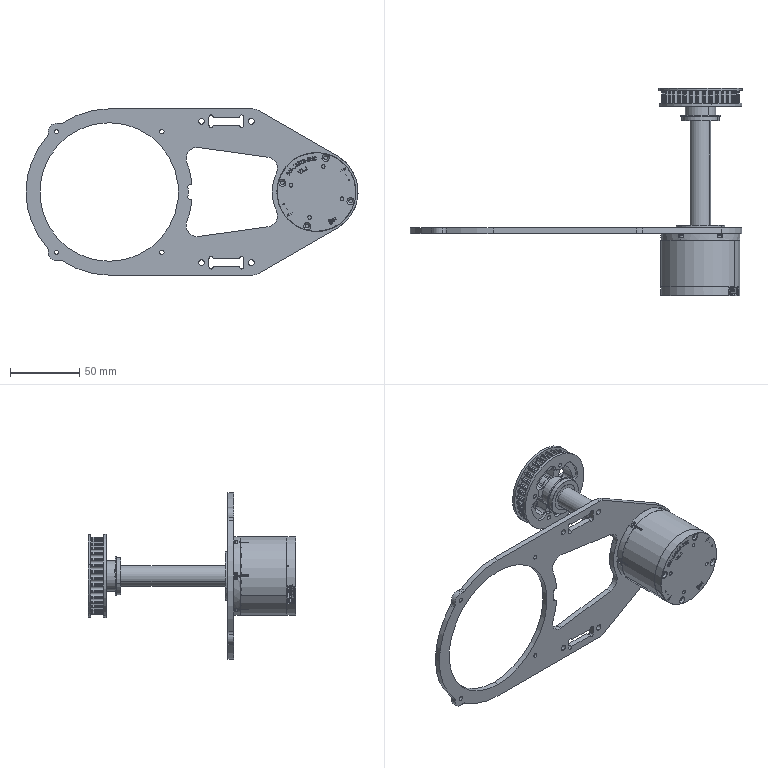Part | SolidWorks | 17 solids | 3464 faces | volume 185614 mm3 | cylinder 1482 | plane 1270 | spline 379 | cone 301 | torus 32 | commonest cylinder face diameters 2.5 x276 2 x253 0.254 x96 0.96 x90 4 x85 3.12 x53